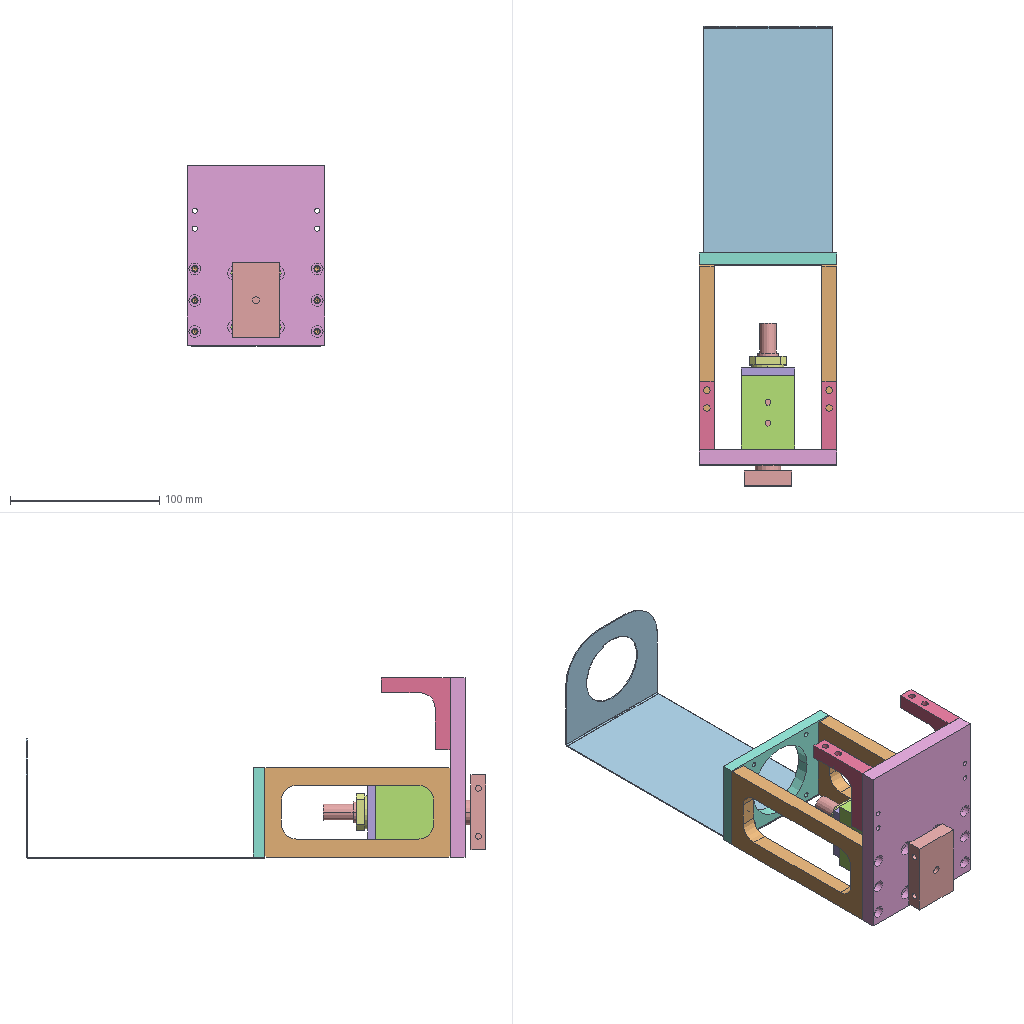Assembly | SolidWorks | 11 different items | 14 placed | box 92 x 308 x 121 mm
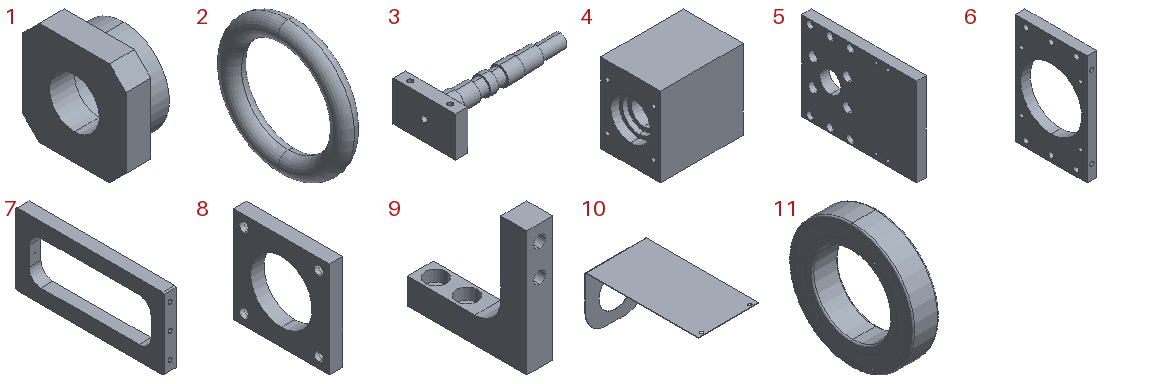Parts list (item | quantity | size | volume | features):
1 | x1 | 13 x 25 x 25 mm | 4305 mm3 | features ICE 2, Chamfer 1, Extrusion 1, HoleWzd 1
2 | x1 | 3 x 20 x 20 mm | 377.512 mm3 | features RefAxis 1, Revolution 1
3 | x1 | 109 x 50 x 32 mm | 28769 mm3 | features ICE 7, RevCut 2, Extrusion 1, RefAxis 1
4 | x1 | 50 x 36 x 48 mm | 72690 mm3 | features ICE 3, HoleWzd 2, Extrusion 1, MirrorPattern 1
5 | x1 | 10 x 120 x 92 mm | 102262 mm3 | features HoleWzd 3, Extrusion 1, ICE 1
6 | x1 | 8 x 60 x 92 mm | 25695 mm3 | features HoleWzd 3, Extrusion 1, ICE 1
7 | x2 | 10 x 124 x 60 mm | 37983 mm3 | features HoleWzd 2, Chamfer 1, Extrusion 1, Fillet 1, ICE 1
8 | x1 | 5 x 36 x 36 mm | 3893 mm3 | features Extrusion 1, HoleWzd 1, ICE 1
9 | x2 | 10 x 46 x 48 mm | 7374 mm3 | features HoleWzd 2, Extrusion 1, Fillet 1, ICE 1
10 | x1 | 86 x 160 x 80 mm | 13487 mm3 | features ICE 2, BreakCorner 1, FlatPattern 1, SMBaseFlange 1, SheetMetal 1
11 | x2 | 5 x 24 x 24 mm | 1358 mm3 | features BaseBody 1
Mates (type | each side: item.copy, entity, surface, feature):
Concentric | 3.1 face cylinder Boss-Extrude3 | 11.1 face cylinder Input1
Coincident | 3.1 face plane Boss-Extrude2 | 11.1 face plane Input1
Concentric | 3.1 face cylinder Boss-Extrude3 | 4.1 face cylinder Boss-Extrude1
Parallel | 3.1 face plane Boss-Extrude1 | 4.1 face plane Boss-Extrude1
Coincident | 3.1 face plane Boss-Extrude2 | 4.1 face plane Boss-Extrude1
Concentric | 3.1 face cylinder Boss-Extrude3 | 11.2 face cylinder Input1
Coincident | 4.1 face plane Cut-Extrude1 | 11.2 face plane Input1
Concentric | 4.1 face cylinder Mirror4 | 5.1 face cylinder Cut-Extrude1
Coincident | 4.1 face plane Boss-Extrude1 | 5.1 face plane Boss-Extrude1
Parallel | 4.1 face plane Boss-Extrude1 | 5.1 face plane Boss-Extrude1
Coincident | 6.1 face plane Boss-Extrude1 | 7.1 face plane Boss-Extrude1 | 3 times
Coincident | 5.1 face plane Boss-Extrude1 | 7.1 face plane Boss-Extrude1
Coincident | 6.1 face plane Boss-Extrude1 | 7.2 face plane Boss-Extrude1 | 3 times
Concentric | 4.1 face cylinder Cut-Extrude1 | 8.1 face cylinder Cut-Extrude2
Coincident | 4.1 face plane Boss-Extrude1 | 8.1 face plane Boss-Extrude1
Parallel | 4.1 face plane Boss-Extrude1 | 8.1 face plane Boss-Extrude1
Concentric | 4.1 face cylinder Cut-Extrude2 | 2.1 select_type:24
DistanceDim | 2.1 plane | 4.1 face plane Cut-Extrude2
Coincident | 5.1 face plane Boss-Extrude1 | 9.1 face plane Boss-Extrude1 | 3 times
Coincident | 5.1 face plane Boss-Extrude1 | 9.2 face plane Boss-Extrude1 | 3 times
Coincident | 6.1 face plane Boss-Extrude1 | 10.1 face plane Base-Flange1 | 2 times
Width | 6.1 face plane Boss-Extrude1 | 6.1 face plane Boss-Extrude1 | 10.1 face plane Base-Flange1 | 10.1 face plane Base-Flange1
Concentric | 3.1 face cylinder Cut-Revolve2 | 1.1 face cylinder Boss-Extrude2
Parallel | 4.1 face plane Boss-Extrude1 | 1.1 face plane Boss-Extrude1
Coincident | 11.2 face plane Input1 | 1.1 face plane Boss-Extrude2